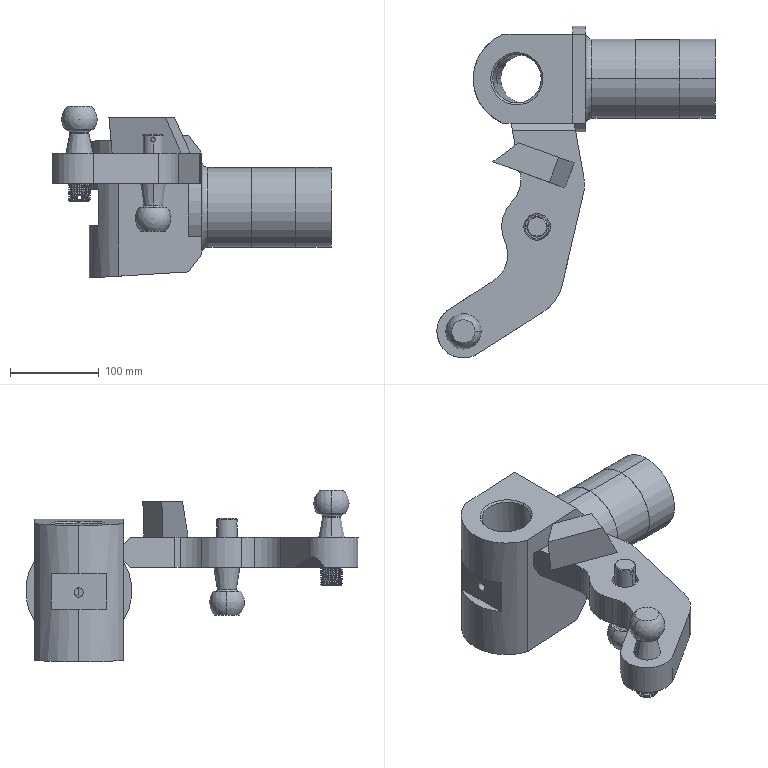Part | SolidWorks | features CompositeCurve 2, AEMSimFeature 1 | 5 solids | 173 faces | box 314 x 375 x 193.9 mm | volume 3181151 mm3 | cylinder 71 | plane 41 | cone 31 | torus 14 | spline 12 | sphere 4 | commonest cylinder face diameters 24 x24 10.5 x14 5 x4 30 x4 70 x4 90 x4